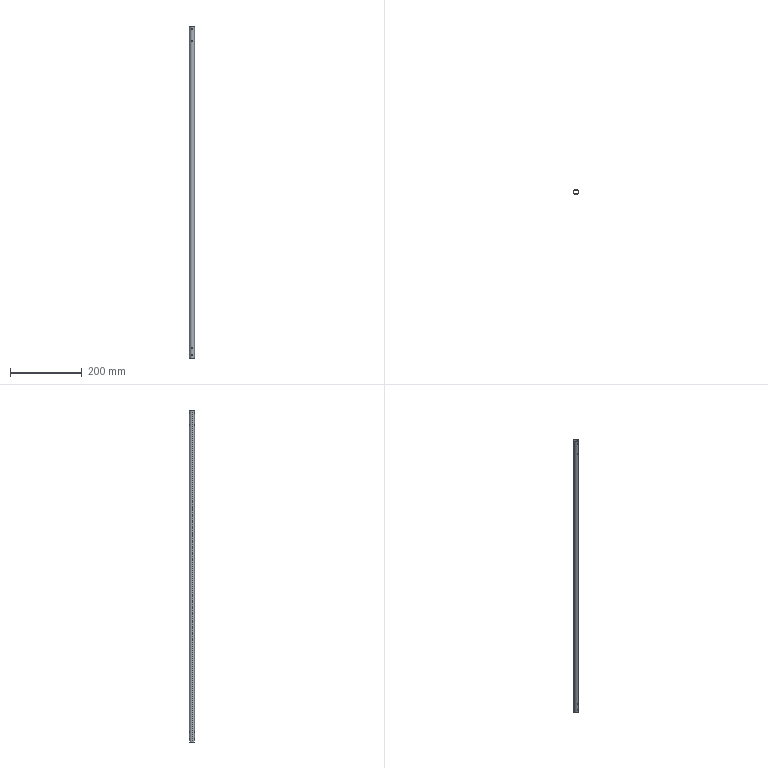Part | SolidWorks | features Extrusion 1, ICE 1 | 1 solid | 22 faces | box 14 x 14 x 926.63 mm | volume 19619 mm3 | cylinder 20 | plane 2 | commonest cylinder face diameters 3.1 x16 13 x2 14 x2